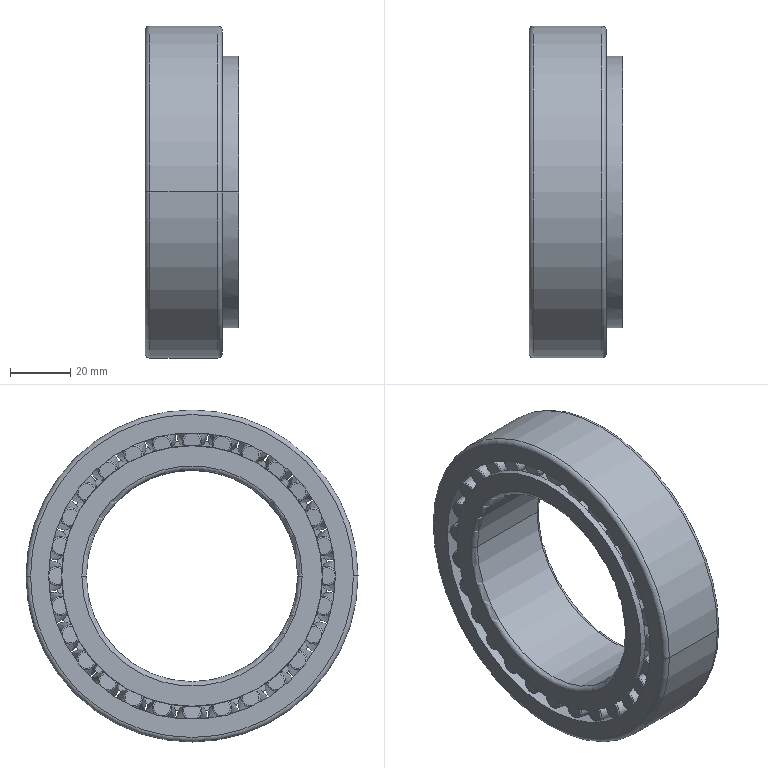Part | SolidWorks | features Revolution 3, CirPattern 1 | 1 solid | 252 faces | box 31 x 110 x 110 mm | volume 131745 mm3 | torus 120 | cone 64 | plane 60 | cylinder 8 | commonest cylinder face diameters 70 x2 86.283 x2 89.854 x2 110 x2